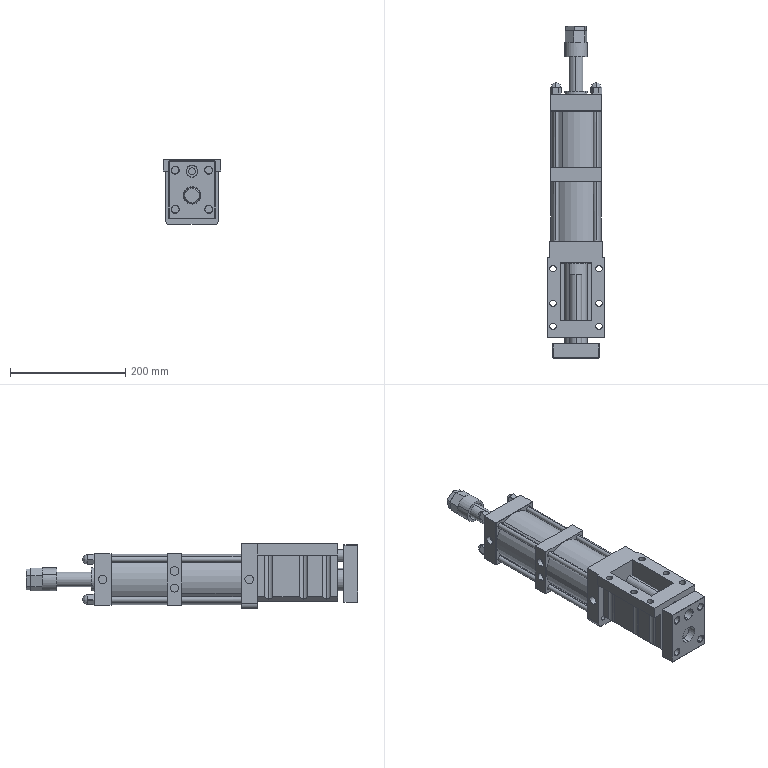Part | SolidWorks | features BaseBody 23, ICE 1 | 23 solids | 831 faces | box 100 x 577.1 x 113 mm | volume 2394119 mm3 | cylinder 500 | plane 227 | spline 54 | cone 50 | commonest cylinder face diameters 8.6 x112 15 x86 9.593 x56 22 x46 11 x28 19.495 x24